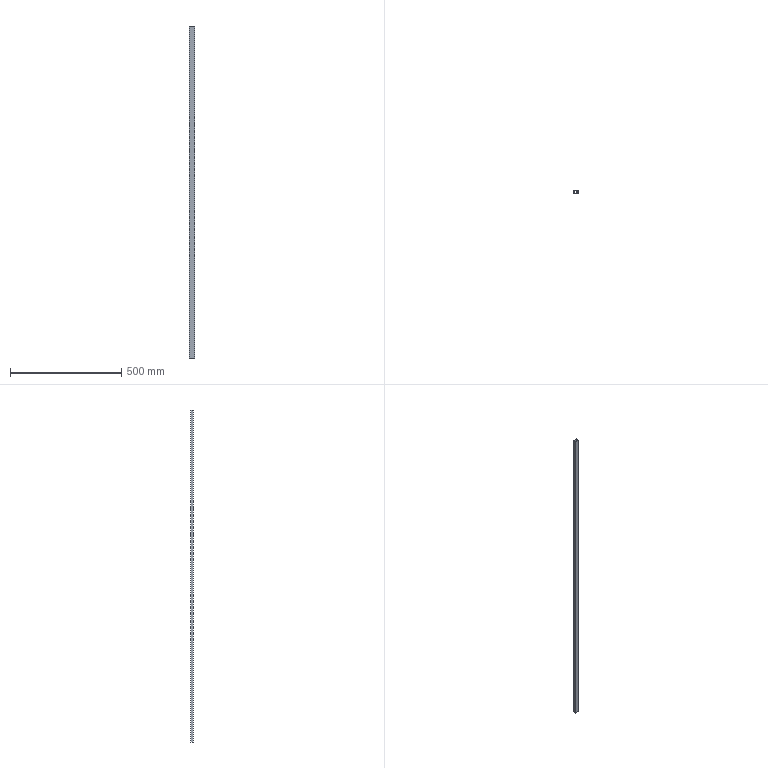Part | SolidWorks | features ExtruThin 1, WeldmentFeature 1 | 1 solid | 10 faces | box 23 x 13 x 1490 mm | volume 147510 mm3 | plane 10
STEP:
#1=CARTESIAN_POINT('',(-1.5,1.5,1490.));
#2=VERTEX_POINT('',#1);
#3=CARTESIAN_POINT('',(-1.5,-11.5,1490.));
#4=VERTEX_POINT('',#3);
#5=CARTESIAN_POINT('',(-1.5,0.,1490.));
#6=DIRECTION('',(0.,-1.,0.));
#7=VECTOR('',#6,1000.);
#8=LINE('',#5,#7);
#9=EDGE_CURVE('',#2,#4,#8,.T.);
#10=ORIENTED_EDGE('',*,*,#9,.T.);
#11=CARTESIAN_POINT('',(21.5,-11.5,1490.));
#12=VERTEX_POINT('',#11);
#13=CARTESIAN_POINT('',(0.,-11.5,1490.));
#14=DIRECTION('',(1.,0.,0.));
#15=VECTOR('',#14,1000.);
#16=LINE('',#13,#15);
#17=EDGE_CURVE('',#4,#12,#16,.T.);
#18=ORIENTED_EDGE('',*,*,#17,.T.);
#19=CARTESIAN_POINT('',(21.5,1.5,1490.));
#20=VERTEX_POINT('',#19);
#21=CARTESIAN_POINT('',(21.5,0.,1490.));
#22=DIRECTION('',(0.,1.,0.));
#23=VECTOR('',#22,1000.);
#24=LINE('',#21,#23);
#25=EDGE_CURVE('',#12,#20,#24,.T.);
#26=ORIENTED_EDGE('',*,*,#25,.T.);
#27=CARTESIAN_POINT('',(0.,1.5,1490.));
#28=DIRECTION('',(-1.,0.,0.));
#29=VECTOR('',#28,1000.);
#30=LINE('',#27,#29);
#31=EDGE_CURVE('',#20,#2,#30,.T.);
#32=ORIENTED_EDGE('',*,*,#31,.T.);
#33=EDGE_LOOP('',(#10,#18,#26,#32));
#34=FACE_OUTER_BOUND('',#33,.T.);
#35=CARTESIAN_POINT('',(0.,-10.,1490.));
#36=VERTEX_POINT('',#35);
#37=CARTESIAN_POINT('',(20.,-10.,1490.));
#38=VERTEX_POINT('',#37);
#39=CARTESIAN_POINT('',(0.,-10.,1490.));
#40=DIRECTION('',(1.,0.,0.));
#41=VECTOR('',#40,1000.);
#42=LINE('',#39,#41);
#43=EDGE_CURVE('',#36,#38,#42,.T.);
#44=ORIENTED_EDGE('',*,*,#43,.F.);
#45=CARTESIAN_POINT('',(0.,0.,1490.));
#46=VERTEX_POINT('',#45);
#47=CARTESIAN_POINT('',(0.,0.,1490.));
#48=DIRECTION('',(0.,-1.,0.));
#49=VECTOR('',#48,1000.);
#50=LINE('',#47,#49);
#51=EDGE_CURVE('',#46,#36,#50,.T.);
#52=ORIENTED_EDGE('',*,*,#51,.F.);
#53=CARTESIAN_POINT('',(20.,0.,1490.));
#54=VERTEX_POINT('',#53);
#55=CARTESIAN_POINT('',(0.,0.,1490.));
#56=DIRECTION('',(-1.,0.,0.));
#57=VECTOR('',#56,1000.);
#58=LINE('',#55,#57);
#59=EDGE_CURVE('',#54,#46,#58,.T.);
#60=ORIENTED_EDGE('',*,*,#59,.F.);
#61=CARTESIAN_POINT('',(20.,0.,1490.));
#62=DIRECTION('',(0.,1.,0.));
#63=VECTOR('',#62,1000.);
#64=LINE('',#61,#63);
#65=EDGE_CURVE('',#38,#54,#64,.T.);
#66=ORIENTED_EDGE('',*,*,#65,.F.);
#67=EDGE_LOOP('',(#44,#52,#60,#66));
#68=FACE_BOUND('',#67,.T.);
#69=CARTESIAN_POINT('',(0.,0.,1490.));
#70=DIRECTION('',(0.,0.,1.));
#71=DIRECTION('',(1.,0.,0.));
#72=AXIS2_PLACEMENT_3D('',#69,#70,#71);
#73=PLANE('',#72);
#74=ADVANCED_FACE('',(#34,#68),#73,.T.);
#75=CARTESIAN_POINT('',(-1.5,1.5,0.));
#76=VERTEX_POINT('',#75);
#77=CARTESIAN_POINT('',(-1.5,-11.5,0.));
#78=VERTEX_POINT('',#77);
#79=CARTESIAN_POINT('',(-1.5,0.,0.));
#80=DIRECTION('',(0.,-1.,0.));
#81=VECTOR('',#80,1000.);
#82=LINE('',#79,#81);
#83=EDGE_CURVE('',#76,#78,#82,.T.);
#84=ORIENTED_EDGE('',*,*,#83,.F.);
#85=CARTESIAN_POINT('',(21.5,1.5,0.));
#86=VERTEX_POINT('',#85);
#87=CARTESIAN_POINT('',(0.,1.5,0.));
#88=DIRECTION('',(-1.,0.,0.));
#89=VECTOR('',#88,1000.);
#90=LINE('',#87,#89);
#91=EDGE_CURVE('',#86,#76,#90,.T.);
#92=ORIENTED_EDGE('',*,*,#91,.F.);
#93=CARTESIAN_POINT('',(21.5,-11.5,0.));
#94=VERTEX_POINT('',#93);
#95=CARTESIAN_POINT('',(21.5,0.,0.));
#96=DIRECTION('',(0.,1.,0.));
#97=VECTOR('',#96,1000.);
#98=LINE('',#95,#97);
#99=EDGE_CURVE('',#94,#86,#98,.T.);
#100=ORIENTED_EDGE('',*,*,#99,.F.);
#101=CARTESIAN_POINT('',(0.,-11.5,0.));
#102=DIRECTION('',(1.,0.,0.));
#103=VECTOR('',#102,1000.);
#104=LINE('',#101,#103);
#105=EDGE_CURVE('',#78,#94,#104,.T.);
#106=ORIENTED_EDGE('',*,*,#105,.F.);
#107=EDGE_LOOP('',(#84,#92,#100,#106));
#108=FACE_OUTER_BOUND('',#107,.T.);
#109=CARTESIAN_POINT('',(0.,0.,0.));
#110=VERTEX_POINT('',#109);
#111=CARTESIAN_POINT('',(0.,-10.,0.));
#112=VERTEX_POINT('',#111);
#113=CARTESIAN_POINT('',(0.,0.,0.));
#114=DIRECTION('',(0.,-1.,0.));
#115=VECTOR('',#114,1000.);
#116=LINE('',#113,#115);
#117=EDGE_CURVE('',#110,#112,#116,.T.);
#118=ORIENTED_EDGE('',*,*,#117,.T.);
#119=CARTESIAN_POINT('',(20.,-10.,0.));
#120=VERTEX_POINT('',#119);
#121=CARTESIAN_POINT('',(0.,-10.,0.));
#122=DIRECTION('',(1.,0.,0.));
#123=VECTOR('',#122,1000.);
#124=LINE('',#121,#123);
#125=EDGE_CURVE('',#112,#120,#124,.T.);
#126=ORIENTED_EDGE('',*,*,#125,.T.);
#127=CARTESIAN_POINT('',(20.,0.,0.));
#128=VERTEX_POINT('',#127);
#129=CARTESIAN_POINT('',(20.,0.,0.));
#130=DIRECTION('',(0.,1.,0.));
#131=VECTOR('',#130,1000.);
#132=LINE('',#129,#131);
#133=EDGE_CURVE('',#120,#128,#132,.T.);
#134=ORIENTED_EDGE('',*,*,#133,.T.);
#135=CARTESIAN_POINT('',(0.,0.,0.));
#136=DIRECTION('',(-1.,0.,0.));
#137=VECTOR('',#136,1000.);
#138=LINE('',#135,#137);
#139=EDGE_CURVE('',#128,#110,#138,.T.);
#140=ORIENTED_EDGE('',*,*,#139,.T.);
#141=EDGE_LOOP('',(#118,#126,#134,#140));
#142=FACE_BOUND('',#141,.T.);
#143=CARTESIAN_POINT('',(0.,0.,0.));
#144=DIRECTION('',(0.,0.,1.));
#145=DIRECTION('',(1.,0.,0.));
#146=AXIS2_PLACEMENT_3D('',#143,#144,#145);
#147=PLANE('',#146);
#148=ADVANCED_FACE('',(#108,#142),#147,.F.);
#149=ORIENTED_EDGE('',*,*,#83,.T.);
#150=CARTESIAN_POINT('',(-1.5,-11.5,1490.));
#151=DIRECTION('',(0.,0.,-1.));
#152=VECTOR('',#151,1000.);
#153=LINE('',#150,#152);
#154=EDGE_CURVE('',#4,#78,#153,.T.);
#155=ORIENTED_EDGE('',*,*,#154,.F.);
#156=ORIENTED_EDGE('',*,*,#9,.F.);
#157=CARTESIAN_POINT('',(-1.5,1.5,1490.));
#158=DIRECTION('',(0.,0.,-1.));
#159=VECTOR('',#158,1000.);
#160=LINE('',#157,#159);
#161=EDGE_CURVE('',#2,#76,#160,.T.);
#162=ORIENTED_EDGE('',*,*,#161,.T.);
#163=EDGE_LOOP('',(#149,#155,#156,#162));
#164=FACE_OUTER_BOUND('',#163,.T.);
#165=CARTESIAN_POINT('',(-1.5,0.,1490.));
#166=DIRECTION('',(1.,0.,0.));
#167=DIRECTION('',(0.,0.,-1.));
#168=AXIS2_PLACEMENT_3D('',#165,#166,#167);
#169=PLANE('',#168);
#170=ADVANCED_FACE('',(#164),#169,.F.);
#171=ORIENTED_EDGE('',*,*,#105,.T.);
#172=CARTESIAN_POINT('',(21.5,-11.5,1490.));
#173=DIRECTION('',(0.,0.,-1.));
#174=VECTOR('',#173,1000.);
#175=LINE('',#172,#174);
#176=EDGE_CURVE('',#12,#94,#175,.T.);
#177=ORIENTED_EDGE('',*,*,#176,.F.);
#178=ORIENTED_EDGE('',*,*,#17,.F.);
#179=ORIENTED_EDGE('',*,*,#154,.T.);
#180=EDGE_LOOP('',(#171,#177,#178,#179));
#181=FACE_OUTER_BOUND('',#180,.T.);
#182=CARTESIAN_POINT('',(0.,-11.5,1490.));
#183=DIRECTION('',(0.,1.,0.));
#184=DIRECTION('',(0.,0.,1.));
#185=AXIS2_PLACEMENT_3D('',#182,#183,#184);
#186=PLANE('',#185);
#187=ADVANCED_FACE('',(#181),#186,.F.);
#188=ORIENTED_EDGE('',*,*,#99,.T.);
#189=CARTESIAN_POINT('',(21.5,1.5,1490.));
#190=DIRECTION('',(0.,0.,-1.));
#191=VECTOR('',#190,1000.);
#192=LINE('',#189,#191);
#193=EDGE_CURVE('',#20,#86,#192,.T.);
#194=ORIENTED_EDGE('',*,*,#193,.F.);
#195=ORIENTED_EDGE('',*,*,#25,.F.);
#196=ORIENTED_EDGE('',*,*,#176,.T.);
#197=EDGE_LOOP('',(#188,#194,#195,#196));
#198=FACE_OUTER_BOUND('',#197,.T.);
#199=CARTESIAN_POINT('',(21.5,0.,1490.));
#200=DIRECTION('',(-1.,0.,0.));
#201=DIRECTION('',(0.,-1.,0.));
#202=AXIS2_PLACEMENT_3D('',#199,#200,#201);
#203=PLANE('',#202);
#204=ADVANCED_FACE('',(#198),#203,.F.);
#205=ORIENTED_EDGE('',*,*,#91,.T.);
#206=ORIENTED_EDGE('',*,*,#161,.F.);
#207=ORIENTED_EDGE('',*,*,#31,.F.);
#208=ORIENTED_EDGE('',*,*,#193,.T.);
#209=EDGE_LOOP('',(#205,#206,#207,#208));
#210=FACE_OUTER_BOUND('',#209,.T.);
#211=CARTESIAN_POINT('',(0.,1.5,1490.));
#212=DIRECTION('',(0.,-1.,0.));
#213=DIRECTION('',(0.,0.,-1.));
#214=AXIS2_PLACEMENT_3D('',#211,#212,#213);
#215=PLANE('',#214);
#216=ADVANCED_FACE('',(#210),#215,.F.);
#217=ORIENTED_EDGE('',*,*,#117,.F.);
#218=CARTESIAN_POINT('',(0.,0.,1490.));
#219=DIRECTION('',(0.,0.,-1.));
#220=VECTOR('',#219,1000.);
#221=LINE('',#218,#220);
#222=EDGE_CURVE('',#46,#110,#221,.T.);
#223=ORIENTED_EDGE('',*,*,#222,.F.);
#224=ORIENTED_EDGE('',*,*,#51,.T.);
#225=CARTESIAN_POINT('',(0.,-10.,1490.));
#226=DIRECTION('',(0.,0.,-1.));
#227=VECTOR('',#226,1000.);
#228=LINE('',#225,#227);
#229=EDGE_CURVE('',#36,#112,#228,.T.);
#230=ORIENTED_EDGE('',*,*,#229,.T.);
#231=EDGE_LOOP('',(#217,#223,#224,#230));
#232=FACE_OUTER_BOUND('',#231,.T.);
#233=CARTESIAN_POINT('',(0.,0.,1490.));
#234=DIRECTION('',(1.,0.,0.));
#235=DIRECTION('',(0.,0.,-1.));
#236=AXIS2_PLACEMENT_3D('',#233,#234,#235);
#237=PLANE('',#236);
#238=ADVANCED_FACE('',(#232),#237,.T.);
#239=ORIENTED_EDGE('',*,*,#125,.F.);
#240=ORIENTED_EDGE('',*,*,#229,.F.);
#241=ORIENTED_EDGE('',*,*,#43,.T.);
#242=CARTESIAN_POINT('',(20.,-10.,1490.));
#243=DIRECTION('',(0.,0.,-1.));
#244=VECTOR('',#243,1000.);
#245=LINE('',#242,#244);
#246=EDGE_CURVE('',#38,#120,#245,.T.);
#247=ORIENTED_EDGE('',*,*,#246,.T.);
#248=EDGE_LOOP('',(#239,#240,#241,#247));
#249=FACE_OUTER_BOUND('',#248,.T.);
#250=CARTESIAN_POINT('',(0.,-10.,1490.));
#251=DIRECTION('',(0.,1.,0.));
#252=DIRECTION('',(0.,0.,1.));
#253=AXIS2_PLACEMENT_3D('',#250,#251,#252);
#254=PLANE('',#253);
#255=ADVANCED_FACE('',(#249),#254,.T.);
#256=ORIENTED_EDGE('',*,*,#133,.F.);
#257=ORIENTED_EDGE('',*,*,#246,.F.);
#258=ORIENTED_EDGE('',*,*,#65,.T.);
#259=CARTESIAN_POINT('',(20.,0.,1490.));
#260=DIRECTION('',(0.,0.,-1.));
#261=VECTOR('',#260,1000.);
#262=LINE('',#259,#261);
#263=EDGE_CURVE('',#54,#128,#262,.T.);
#264=ORIENTED_EDGE('',*,*,#263,.T.);
#265=EDGE_LOOP('',(#256,#257,#258,#264));
#266=FACE_OUTER_BOUND('',#265,.T.);
#267=CARTESIAN_POINT('',(20.,0.,1490.));
#268=DIRECTION('',(-1.,0.,0.));
#269=DIRECTION('',(0.,-1.,0.));
#270=AXIS2_PLACEMENT_3D('',#267,#268,#269);
#271=PLANE('',#270);
#272=ADVANCED_FACE('',(#266),#271,.T.);
#273=ORIENTED_EDGE('',*,*,#139,.F.);
#274=ORIENTED_EDGE('',*,*,#263,.F.);
#275=ORIENTED_EDGE('',*,*,#59,.T.);
#276=ORIENTED_EDGE('',*,*,#222,.T.);
#277=EDGE_LOOP('',(#273,#274,#275,#276));
#278=FACE_OUTER_BOUND('',#277,.T.);
#279=CARTESIAN_POINT('',(0.,0.,1490.));
#280=DIRECTION('',(0.,-1.,0.));
#281=DIRECTION('',(0.,0.,-1.));
#282=AXIS2_PLACEMENT_3D('',#279,#280,#281);
#283=PLANE('',#282);
#284=ADVANCED_FACE('',(#278),#283,.T.);
#285=CLOSED_SHELL('',(#74,#148,#170,#187,#204,#216,#238,#255,#272,#284));
#286=MANIFOLD_SOLID_BREP('',#285);
#287=CARTESIAN_POINT('',(0.,0.,0.));
#288=DIRECTION('',(0.,0.,1.));
#289=DIRECTION('',(1.,0.,0.));
#290=AXIS2_PLACEMENT_3D('',#287,#288,#289);
#291=(LENGTH_UNIT()NAMED_UNIT(*)SI_UNIT(.MILLI.,.METRE.));
#292=UNCERTAINTY_MEASURE_WITH_UNIT(LENGTH_MEASURE(0.00001),#291,'','');
#293=(NAMED_UNIT(*)PLANE_ANGLE_UNIT()SI_UNIT($,.RADIAN.));
#294=(NAMED_UNIT(*)SI_UNIT($,.STERADIAN.)SOLID_ANGLE_UNIT());
#295=(GEOMETRIC_REPRESENTATION_CONTEXT(3)GLOBAL_UNCERTAINTY_ASSIGNED_CONTEXT((#292))GLOBAL_UNIT_ASSIGNED_CONTEXT((#291,#293,#294))REPRESENTATION_CONTEXT('',''));
#296=ADVANCED_BREP_SHAPE_REPRESENTATION('',(#286,#290),#295);